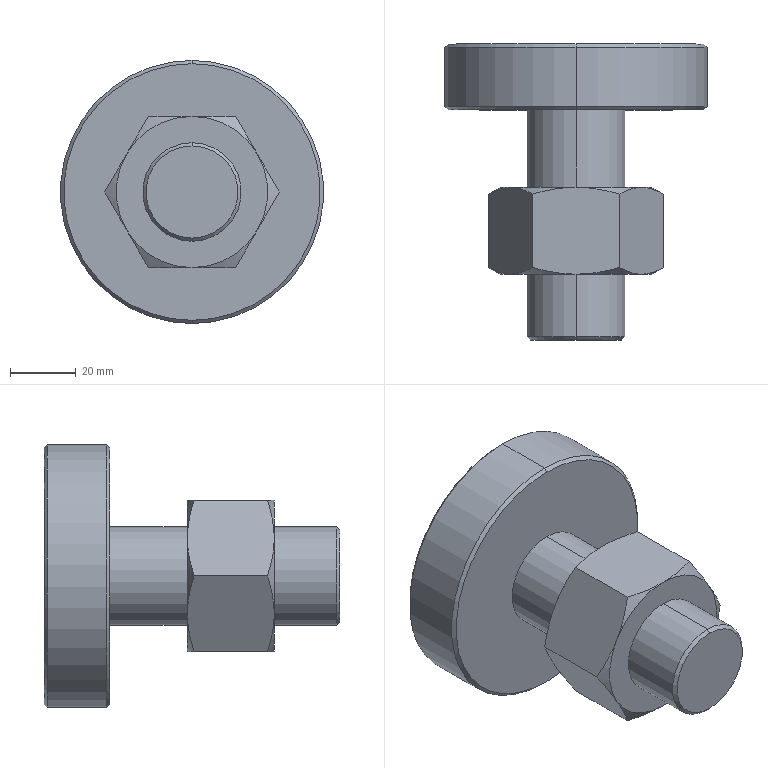Part | SolidWorks | features BaseBody 2 | 2 solids | 35 faces | box 80 x 90 x 80 mm | volume 179222 mm3 | cone 18 | plane 11 | cylinder 6 | commonest cylinder face diameters 30 x4 80 x2
STEP:
#1=CARTESIAN_POINT('',(0.,-70.,-14.));
#2=VERTEX_POINT('',#1);
#3=CARTESIAN_POINT('',(0.,-70.,14.));
#4=VERTEX_POINT('',#3);
#5=CARTESIAN_POINT('',(0.,-70.,0.));
#6=DIRECTION('',(0.,-1.,0.));
#7=DIRECTION('',(0.,0.,1.));
#8=AXIS2_PLACEMENT_3D('',#5,#6,#7);
#9=CIRCLE('',#8,14.);
#10=EDGE_CURVE('',#2,#4,#9,.T.);
#11=ORIENTED_EDGE('',*,*,#10,.F.);
#12=CARTESIAN_POINT('',(0.,-69.,-15.));
#13=VERTEX_POINT('',#12);
#14=CARTESIAN_POINT('',(0.,-69.,-15.));
#15=DIRECTION('',(0.,0.7071,-0.7071));
#16=VECTOR('',#15,1000.);
#17=LINE('',#14,#16);
#18=EDGE_CURVE('',#2,#13,#17,.T.);
#19=ORIENTED_EDGE('',*,*,#18,.T.);
#20=CARTESIAN_POINT('',(0.,-69.,15.));
#21=VERTEX_POINT('',#20);
#22=CARTESIAN_POINT('',(0.,-69.,0.));
#23=DIRECTION('',(0.,1.,0.));
#24=DIRECTION('',(0.,0.,1.));
#25=AXIS2_PLACEMENT_3D('',#22,#23,#24);
#26=CIRCLE('',#25,15.);
#27=EDGE_CURVE('',#21,#13,#26,.T.);
#28=ORIENTED_EDGE('',*,*,#27,.F.);
#29=CARTESIAN_POINT('',(0.,-69.,15.));
#30=DIRECTION('',(0.,0.7071,0.7071));
#31=VECTOR('',#30,1000.);
#32=LINE('',#29,#31);
#33=EDGE_CURVE('',#4,#21,#32,.T.);
#34=ORIENTED_EDGE('',*,*,#33,.F.);
#35=EDGE_LOOP('',(#11,#19,#28,#34));
#36=FACE_OUTER_BOUND('',#35,.T.);
#37=CARTESIAN_POINT('',(0.,-69.,0.));
#38=DIRECTION('',(0.,1.,0.));
#39=DIRECTION('',(0.,0.,1.));
#40=AXIS2_PLACEMENT_3D('',#37,#38,#39);
#41=CONICAL_SURFACE('',#40,15.,0.7854);
#42=ADVANCED_FACE('',(#36),#41,.T.);
#43=CARTESIAN_POINT('',(0.,0.,-39.));
#44=VERTEX_POINT('',#43);
#45=CARTESIAN_POINT('',(0.,0.,39.));
#46=VERTEX_POINT('',#45);
#47=CARTESIAN_POINT('',(0.,0.,0.));
#48=DIRECTION('',(0.,-1.,0.));
#49=DIRECTION('',(0.,0.,1.));
#50=AXIS2_PLACEMENT_3D('',#47,#48,#49);
#51=CIRCLE('',#50,39.);
#52=EDGE_CURVE('',#44,#46,#51,.T.);
#53=ORIENTED_EDGE('',*,*,#52,.F.);
#54=CARTESIAN_POINT('',(0.,1.,-40.));
#55=VERTEX_POINT('',#54);
#56=CARTESIAN_POINT('',(0.,1.,-40.));
#57=DIRECTION('',(0.,0.7071,-0.7071));
#58=VECTOR('',#57,1000.);
#59=LINE('',#56,#58);
#60=EDGE_CURVE('',#44,#55,#59,.T.);
#61=ORIENTED_EDGE('',*,*,#60,.T.);
#62=CARTESIAN_POINT('',(0.,1.,40.));
#63=VERTEX_POINT('',#62);
#64=CARTESIAN_POINT('',(0.,1.,0.));
#65=DIRECTION('',(0.,1.,0.));
#66=DIRECTION('',(0.,0.,1.));
#67=AXIS2_PLACEMENT_3D('',#64,#65,#66);
#68=CIRCLE('',#67,40.);
#69=EDGE_CURVE('',#63,#55,#68,.T.);
#70=ORIENTED_EDGE('',*,*,#69,.F.);
#71=CARTESIAN_POINT('',(0.,1.,40.));
#72=DIRECTION('',(0.,0.7071,0.7071));
#73=VECTOR('',#72,1000.);
#74=LINE('',#71,#73);
#75=EDGE_CURVE('',#46,#63,#74,.T.);
#76=ORIENTED_EDGE('',*,*,#75,.F.);
#77=EDGE_LOOP('',(#53,#61,#70,#76));
#78=FACE_OUTER_BOUND('',#77,.T.);
#79=CARTESIAN_POINT('',(0.,1.,0.));
#80=DIRECTION('',(0.,1.,0.));
#81=DIRECTION('',(0.,0.,1.));
#82=AXIS2_PLACEMENT_3D('',#79,#80,#81);
#83=CONICAL_SURFACE('',#82,40.,0.7854);
#84=ADVANCED_FACE('',(#78),#83,.T.);
#85=CARTESIAN_POINT('',(0.,20.,39.));
#86=VERTEX_POINT('',#85);
#87=CARTESIAN_POINT('',(0.,20.,-39.));
#88=VERTEX_POINT('',#87);
#89=CARTESIAN_POINT('',(0.,20.,0.));
#90=DIRECTION('',(0.,1.,0.));
#91=DIRECTION('',(0.,0.,1.));
#92=AXIS2_PLACEMENT_3D('',#89,#90,#91);
#93=CIRCLE('',#92,39.);
#94=EDGE_CURVE('',#86,#88,#93,.T.);
#95=ORIENTED_EDGE('',*,*,#94,.F.);
#96=CARTESIAN_POINT('',(0.,19.,40.));
#97=VERTEX_POINT('',#96);
#98=CARTESIAN_POINT('',(0.,20.,39.));
#99=DIRECTION('',(0.,-0.7071,0.7071));
#100=VECTOR('',#99,1000.);
#101=LINE('',#98,#100);
#102=EDGE_CURVE('',#86,#97,#101,.T.);
#103=ORIENTED_EDGE('',*,*,#102,.T.);
#104=CARTESIAN_POINT('',(0.,19.,-40.));
#105=VERTEX_POINT('',#104);
#106=CARTESIAN_POINT('',(0.,19.,0.));
#107=DIRECTION('',(0.,-1.,0.));
#108=DIRECTION('',(0.,0.,1.));
#109=AXIS2_PLACEMENT_3D('',#106,#107,#108);
#110=CIRCLE('',#109,40.);
#111=EDGE_CURVE('',#105,#97,#110,.T.);
#112=ORIENTED_EDGE('',*,*,#111,.F.);
#113=CARTESIAN_POINT('',(0.,20.,-39.));
#114=DIRECTION('',(0.,-0.7071,-0.7071));
#115=VECTOR('',#114,1000.);
#116=LINE('',#113,#115);
#117=EDGE_CURVE('',#88,#105,#116,.T.);
#118=ORIENTED_EDGE('',*,*,#117,.F.);
#119=EDGE_LOOP('',(#95,#103,#112,#118));
#120=FACE_OUTER_BOUND('',#119,.T.);
#121=CARTESIAN_POINT('',(0.,20.,0.));
#122=DIRECTION('',(0.,-1.,0.));
#123=DIRECTION('',(0.,0.,-1.));
#124=AXIS2_PLACEMENT_3D('',#121,#122,#123);
#125=CONICAL_SURFACE('',#124,39.,0.7854);
#126=ADVANCED_FACE('',(#120),#125,.T.);
#127=ORIENTED_EDGE('',*,*,#27,.T.);
#128=CARTESIAN_POINT('',(0.,0.,-15.));
#129=VERTEX_POINT('',#128);
#130=CARTESIAN_POINT('',(0.,-70.,-15.));
#131=DIRECTION('',(0.,1.,0.));
#132=VECTOR('',#131,1000.);
#133=LINE('',#130,#132);
#134=EDGE_CURVE('',#13,#129,#133,.T.);
#135=ORIENTED_EDGE('',*,*,#134,.T.);
#136=CARTESIAN_POINT('',(0.,0.,15.));
#137=VERTEX_POINT('',#136);
#138=CARTESIAN_POINT('',(0.,0.,0.));
#139=DIRECTION('',(0.,1.,0.));
#140=DIRECTION('',(0.,0.,1.));
#141=AXIS2_PLACEMENT_3D('',#138,#139,#140);
#142=CIRCLE('',#141,15.);
#143=EDGE_CURVE('',#137,#129,#142,.T.);
#144=ORIENTED_EDGE('',*,*,#143,.F.);
#145=CARTESIAN_POINT('',(0.,-70.,15.));
#146=DIRECTION('',(0.,1.,0.));
#147=VECTOR('',#146,1000.);
#148=LINE('',#145,#147);
#149=EDGE_CURVE('',#21,#137,#148,.T.);
#150=ORIENTED_EDGE('',*,*,#149,.F.);
#151=EDGE_LOOP('',(#127,#135,#144,#150));
#152=FACE_OUTER_BOUND('',#151,.T.);
#153=CARTESIAN_POINT('',(0.,-70.,0.));
#154=DIRECTION('',(0.,1.,0.));
#155=DIRECTION('',(0.,0.,1.));
#156=AXIS2_PLACEMENT_3D('',#153,#154,#155);
#157=CYLINDRICAL_SURFACE('',#156,15.);
#158=ADVANCED_FACE('',(#152),#157,.T.);
#159=ORIENTED_EDGE('',*,*,#111,.T.);
#160=CARTESIAN_POINT('',(0.,20.,40.));
#161=DIRECTION('',(0.,-1.,0.));
#162=VECTOR('',#161,1000.);
#163=LINE('',#160,#162);
#164=EDGE_CURVE('',#97,#63,#163,.T.);
#165=ORIENTED_EDGE('',*,*,#164,.T.);
#166=ORIENTED_EDGE('',*,*,#69,.T.);
#167=CARTESIAN_POINT('',(0.,20.,-40.));
#168=DIRECTION('',(0.,-1.,0.));
#169=VECTOR('',#168,1000.);
#170=LINE('',#167,#169);
#171=EDGE_CURVE('',#105,#55,#170,.T.);
#172=ORIENTED_EDGE('',*,*,#171,.F.);
#173=EDGE_LOOP('',(#159,#165,#166,#172));
#174=FACE_OUTER_BOUND('',#173,.T.);
#175=CARTESIAN_POINT('',(0.,20.,0.));
#176=DIRECTION('',(0.,-1.,0.));
#177=DIRECTION('',(0.,0.,-1.));
#178=AXIS2_PLACEMENT_3D('',#175,#176,#177);
#179=CYLINDRICAL_SURFACE('',#178,40.);
#180=ADVANCED_FACE('',(#174),#179,.T.);
#181=CARTESIAN_POINT('',(0.,20.,0.));
#182=DIRECTION('',(0.,1.,0.));
#183=DIRECTION('',(0.,0.,1.));
#184=AXIS2_PLACEMENT_3D('',#181,#182,#183);
#185=CIRCLE('',#184,39.);
#186=EDGE_CURVE('',#88,#86,#185,.T.);
#187=ORIENTED_EDGE('',*,*,#186,.T.);
#188=ORIENTED_EDGE('',*,*,#94,.T.);
#189=EDGE_LOOP('',(#187,#188));
#190=FACE_OUTER_BOUND('',#189,.T.);
#191=CARTESIAN_POINT('',(0.,20.,0.));
#192=DIRECTION('',(0.,1.,0.));
#193=DIRECTION('',(0.,0.,1.));
#194=AXIS2_PLACEMENT_3D('',#191,#192,#193);
#195=PLANE('',#194);
#196=ADVANCED_FACE('',(#190),#195,.T.);
#197=CARTESIAN_POINT('',(0.,0.,0.));
#198=DIRECTION('',(0.,-1.,0.));
#199=DIRECTION('',(0.,0.,1.));
#200=AXIS2_PLACEMENT_3D('',#197,#198,#199);
#201=CIRCLE('',#200,39.);
#202=EDGE_CURVE('',#46,#44,#201,.T.);
#203=ORIENTED_EDGE('',*,*,#202,.T.);
#204=ORIENTED_EDGE('',*,*,#52,.T.);
#205=EDGE_LOOP('',(#203,#204));
#206=FACE_OUTER_BOUND('',#205,.T.);
#207=ORIENTED_EDGE('',*,*,#143,.T.);
#208=CARTESIAN_POINT('',(0.,0.,0.));
#209=DIRECTION('',(0.,1.,0.));
#210=DIRECTION('',(0.,0.,1.));
#211=AXIS2_PLACEMENT_3D('',#208,#209,#210);
#212=CIRCLE('',#211,15.);
#213=EDGE_CURVE('',#129,#137,#212,.T.);
#214=ORIENTED_EDGE('',*,*,#213,.T.);
#215=EDGE_LOOP('',(#207,#214));
#216=FACE_BOUND('',#215,.T.);
#217=CARTESIAN_POINT('',(0.,0.,0.));
#218=DIRECTION('',(0.,1.,0.));
#219=DIRECTION('',(0.,0.,1.));
#220=AXIS2_PLACEMENT_3D('',#217,#218,#219);
#221=PLANE('',#220);
#222=ADVANCED_FACE('',(#206,#216),#221,.F.);
#223=ORIENTED_EDGE('',*,*,#164,.F.);
#224=CARTESIAN_POINT('',(0.,19.,0.));
#225=DIRECTION('',(0.,-1.,0.));
#226=DIRECTION('',(0.,0.,1.));
#227=AXIS2_PLACEMENT_3D('',#224,#225,#226);
#228=CIRCLE('',#227,40.);
#229=EDGE_CURVE('',#97,#105,#228,.T.);
#230=ORIENTED_EDGE('',*,*,#229,.T.);
#231=ORIENTED_EDGE('',*,*,#171,.T.);
#232=CARTESIAN_POINT('',(0.,1.,0.));
#233=DIRECTION('',(0.,1.,0.));
#234=DIRECTION('',(0.,0.,1.));
#235=AXIS2_PLACEMENT_3D('',#232,#233,#234);
#236=CIRCLE('',#235,40.);
#237=EDGE_CURVE('',#55,#63,#236,.T.);
#238=ORIENTED_EDGE('',*,*,#237,.T.);
#239=EDGE_LOOP('',(#223,#230,#231,#238));
#240=FACE_OUTER_BOUND('',#239,.T.);
#241=CARTESIAN_POINT('',(0.,20.,0.));
#242=DIRECTION('',(0.,-1.,0.));
#243=DIRECTION('',(0.,0.,-1.));
#244=AXIS2_PLACEMENT_3D('',#241,#242,#243);
#245=CYLINDRICAL_SURFACE('',#244,40.);
#246=ADVANCED_FACE('',(#240),#245,.T.);
#247=ORIENTED_EDGE('',*,*,#134,.F.);
#248=CARTESIAN_POINT('',(0.,-69.,0.));
#249=DIRECTION('',(0.,1.,0.));
#250=DIRECTION('',(0.,0.,1.));
#251=AXIS2_PLACEMENT_3D('',#248,#249,#250);
#252=CIRCLE('',#251,15.);
#253=EDGE_CURVE('',#13,#21,#252,.T.);
#254=ORIENTED_EDGE('',*,*,#253,.T.);
#255=ORIENTED_EDGE('',*,*,#149,.T.);
#256=ORIENTED_EDGE('',*,*,#213,.F.);
#257=EDGE_LOOP('',(#247,#254,#255,#256));
#258=FACE_OUTER_BOUND('',#257,.T.);
#259=CARTESIAN_POINT('',(0.,-70.,0.));
#260=DIRECTION('',(0.,1.,0.));
#261=DIRECTION('',(0.,0.,1.));
#262=AXIS2_PLACEMENT_3D('',#259,#260,#261);
#263=CYLINDRICAL_SURFACE('',#262,15.);
#264=ADVANCED_FACE('',(#258),#263,.T.);
#265=CARTESIAN_POINT('',(0.,-70.,0.));
#266=DIRECTION('',(0.,-1.,0.));
#267=DIRECTION('',(0.,0.,1.));
#268=AXIS2_PLACEMENT_3D('',#265,#266,#267);
#269=CIRCLE('',#268,14.);
#270=EDGE_CURVE('',#4,#2,#269,.T.);
#271=ORIENTED_EDGE('',*,*,#270,.T.);
#272=ORIENTED_EDGE('',*,*,#10,.T.);
#273=EDGE_LOOP('',(#271,#272));
#274=FACE_OUTER_BOUND('',#273,.T.);
#275=CARTESIAN_POINT('',(0.,-70.,0.));
#276=DIRECTION('',(0.,1.,0.));
#277=DIRECTION('',(0.,0.,1.));
#278=AXIS2_PLACEMENT_3D('',#275,#276,#277);
#279=PLANE('',#278);
#280=ADVANCED_FACE('',(#274),#279,.F.);
#281=ORIENTED_EDGE('',*,*,#102,.F.);
#282=ORIENTED_EDGE('',*,*,#186,.F.);
#283=ORIENTED_EDGE('',*,*,#117,.T.);
#284=ORIENTED_EDGE('',*,*,#229,.F.);
#285=EDGE_LOOP('',(#281,#282,#283,#284));
#286=FACE_OUTER_BOUND('',#285,.T.);
#287=CARTESIAN_POINT('',(0.,20.,0.));
#288=DIRECTION('',(0.,-1.,0.));
#289=DIRECTION('',(0.,0.,-1.));
#290=AXIS2_PLACEMENT_3D('',#287,#288,#289);
#291=CONICAL_SURFACE('',#290,39.,0.7854);
#292=ADVANCED_FACE('',(#286),#291,.T.);
#293=ORIENTED_EDGE('',*,*,#60,.F.);
#294=ORIENTED_EDGE('',*,*,#202,.F.);
#295=ORIENTED_EDGE('',*,*,#75,.T.);
#296=ORIENTED_EDGE('',*,*,#237,.F.);
#297=EDGE_LOOP('',(#293,#294,#295,#296));
#298=FACE_OUTER_BOUND('',#297,.T.);
#299=CARTESIAN_POINT('',(0.,1.,0.));
#300=DIRECTION('',(0.,1.,0.));
#301=DIRECTION('',(0.,0.,1.));
#302=AXIS2_PLACEMENT_3D('',#299,#300,#301);
#303=CONICAL_SURFACE('',#302,40.,0.7854);
#304=ADVANCED_FACE('',(#298),#303,.T.);
#305=ORIENTED_EDGE('',*,*,#18,.F.);
#306=ORIENTED_EDGE('',*,*,#270,.F.);
#307=ORIENTED_EDGE('',*,*,#33,.T.);
#308=ORIENTED_EDGE('',*,*,#253,.F.);
#309=EDGE_LOOP('',(#305,#306,#307,#308));
#310=FACE_OUTER_BOUND('',#309,.T.);
#311=CARTESIAN_POINT('',(0.,-69.,0.));
#312=DIRECTION('',(0.,1.,0.));
#313=DIRECTION('',(0.,0.,1.));
#314=AXIS2_PLACEMENT_3D('',#311,#312,#313);
#315=CONICAL_SURFACE('',#314,15.,0.7854);
#316=ADVANCED_FACE('',(#310),#315,.T.);
#317=CLOSED_SHELL('',(#42,#84,#126,#158,#180,#196,#222,#246,#264,#280,#292,#304,#316));
#318=MANIFOLD_SOLID_BREP('',#317);
#319=CARTESIAN_POINT('',(0.,-23.6,-15.));
#320=VERTEX_POINT('',#319);
#321=CARTESIAN_POINT('',(0.,-23.6,15.));
#322=VERTEX_POINT('',#321);
#323=CARTESIAN_POINT('',(0.,-23.6,0.));
#324=DIRECTION('',(0.,1.,0.));
#325=DIRECTION('',(0.,0.,1.));
#326=AXIS2_PLACEMENT_3D('',#323,#324,#325);
#327=CIRCLE('',#326,15.);
#328=EDGE_CURVE('',#320,#322,#327,.T.);
#329=ORIENTED_EDGE('',*,*,#328,.T.);
#330=CARTESIAN_POINT('',(0.,-50.,15.));
#331=VERTEX_POINT('',#330);
#332=CARTESIAN_POINT('',(0.,-23.6,15.));
#333=DIRECTION('',(0.,-1.,0.));
#334=VECTOR('',#333,1000.);
#335=LINE('',#332,#334);
#336=EDGE_CURVE('',#322,#331,#335,.T.);
#337=ORIENTED_EDGE('',*,*,#336,.T.);
#338=CARTESIAN_POINT('',(0.,-50.,-15.));
#339=VERTEX_POINT('',#338);
#340=CARTESIAN_POINT('',(0.,-50.,0.));
#341=DIRECTION('',(0.,1.,0.));
#342=DIRECTION('',(0.,0.,1.));
#343=AXIS2_PLACEMENT_3D('',#340,#341,#342);
#344=CIRCLE('',#343,15.);
#345=EDGE_CURVE('',#339,#331,#344,.T.);
#346=ORIENTED_EDGE('',*,*,#345,.F.);
#347=CARTESIAN_POINT('',(0.,-23.6,-15.));
#348=DIRECTION('',(0.,-1.,0.));
#349=VECTOR('',#348,1000.);
#350=LINE('',#347,#349);
#351=EDGE_CURVE('',#320,#339,#350,.T.);
#352=ORIENTED_EDGE('',*,*,#351,.F.);
#353=EDGE_LOOP('',(#329,#337,#346,#352));
#354=FACE_OUTER_BOUND('',#353,.T.);
#355=CARTESIAN_POINT('',(0.,-23.6,0.));
#356=DIRECTION('',(0.,-1.,0.));
#357=DIRECTION('',(0.,0.,-1.));
#358=AXIS2_PLACEMENT_3D('',#355,#356,#357);
#359=CYLINDRICAL_SURFACE('',#358,15.);
#360=ADVANCED_FACE('',(#354),#359,.F.);
#361=ORIENTED_EDGE('',*,*,#328,.F.);
#362=CARTESIAN_POINT('',(0.,-23.6,0.));
#363=DIRECTION('',(0.,1.,0.));
#364=DIRECTION('',(0.,0.,1.));
#365=AXIS2_PLACEMENT_3D('',#362,#363,#364);
#366=CIRCLE('',#365,15.);
#367=EDGE_CURVE('',#322,#320,#366,.T.);
#368=ORIENTED_EDGE('',*,*,#367,.F.);
#369=EDGE_LOOP('',(#361,#368));
#370=FACE_BOUND('',#369,.T.);
#371=CARTESIAN_POINT('',(0.,-23.6,23.));
#372=VERTEX_POINT('',#371);
#373=CARTESIAN_POINT('',(-19.919,-23.6,11.5));
#374=VERTEX_POINT('',#373);
#375=CARTESIAN_POINT('',(0.,-23.6,0.));
#376=DIRECTION('',(0.,-1.,0.));
#377=DIRECTION('',(0.,0.,1.));
#378=AXIS2_PLACEMENT_3D('',#375,#376,#377);
#379=CIRCLE('',#378,23.);
#380=EDGE_CURVE('',#372,#374,#379,.T.);
#381=ORIENTED_EDGE('',*,*,#380,.F.);
#382=CARTESIAN_POINT('',(19.919,-23.6,11.5));
#383=VERTEX_POINT('',#382);
#384=CARTESIAN_POINT('',(0.,-23.6,0.));
#385=DIRECTION('',(0.,-1.,0.));
#386=DIRECTION('',(0.,0.,1.));
#387=AXIS2_PLACEMENT_3D('',#384,#385,#386);
#388=CIRCLE('',#387,23.);
#389=EDGE_CURVE('',#383,#372,#388,.T.);
#390=ORIENTED_EDGE('',*,*,#389,.F.);
#391=CARTESIAN_POINT('',(19.919,-23.6,-11.5));
#392=VERTEX_POINT('',#391);
#393=CARTESIAN_POINT('',(0.,-23.6,0.));
#394=DIRECTION('',(0.,-1.,0.));
#395=DIRECTION('',(0.,0.,1.));
#396=AXIS2_PLACEMENT_3D('',#393,#394,#395);
#397=CIRCLE('',#396,23.);
#398=EDGE_CURVE('',#392,#383,#397,.T.);
#399=ORIENTED_EDGE('',*,*,#398,.F.);
#400=CARTESIAN_POINT('',(0.,-23.6,-23.));
#401=VERTEX_POINT('',#400);
#402=CARTESIAN_POINT('',(0.,-23.6,0.));
#403=DIRECTION('',(0.,-1.,0.));
#404=DIRECTION('',(0.,0.,-1.));
#405=AXIS2_PLACEMENT_3D('',#402,#403,#404);
#406=CIRCLE('',#405,23.);
#407=EDGE_CURVE('',#401,#392,#406,.T.);
#408=ORIENTED_EDGE('',*,*,#407,.F.);
#409=CARTESIAN_POINT('',(-19.919,-23.6,-11.5));
#410=VERTEX_POINT('',#409);
#411=CARTESIAN_POINT('',(0.,-23.6,0.));
#412=DIRECTION('',(0.,-1.,0.));
#413=DIRECTION('',(0.,0.,1.));
#414=AXIS2_PLACEMENT_3D('',#411,#412,#413);
#415=CIRCLE('',#414,23.);
#416=EDGE_CURVE('',#410,#401,#415,.T.);
#417=ORIENTED_EDGE('',*,*,#416,.F.);
#418=CARTESIAN_POINT('',(0.,-23.6,0.));
#419=DIRECTION('',(0.,-1.,0.));
#420=DIRECTION('',(0.,0.,1.));
#421=AXIS2_PLACEMENT_3D('',#418,#419,#420);
#422=CIRCLE('',#421,23.);
#423=EDGE_CURVE('',#374,#410,#422,.T.);
#424=ORIENTED_EDGE('',*,*,#423,.F.);
#425=EDGE_LOOP('',(#381,#390,#399,#408,#417,#424));
#426=FACE_OUTER_BOUND('',#425,.T.);
#427=CARTESIAN_POINT('',(0.,-23.6,0.));
#428=DIRECTION('',(0.,1.,0.));
#429=DIRECTION('',(0.,0.,1.));
#430=AXIS2_PLACEMENT_3D('',#427,#428,#429);
#431=PLANE('',#430);
#432=ADVANCED_FACE('',(#370,#426),#431,.T.);
#433=ORIENTED_EDGE('',*,*,#345,.T.);
#434=CARTESIAN_POINT('',(0.,-50.,0.));
#435=DIRECTION('',(0.,1.,0.));
#436=DIRECTION('',(0.,0.,1.));
#437=AXIS2_PLACEMENT_3D('',#434,#435,#436);
#438=CIRCLE('',#437,15.);
#439=EDGE_CURVE('',#331,#339,#438,.T.);
#440=ORIENTED_EDGE('',*,*,#439,.T.);
#441=EDGE_LOOP('',(#433,#440));
#442=FACE_BOUND('',#441,.T.);
#443=CARTESIAN_POINT('',(19.919,-50.,11.5));
#444=VERTEX_POINT('',#443);
#445=CARTESIAN_POINT('',(0.,-50.,23.));
#446=VERTEX_POINT('',#445);
#447=CARTESIAN_POINT('',(0.,-50.,0.));
#448=DIRECTION('',(0.,-1.,0.));
#449=DIRECTION('',(0.,0.,-1.));
#450=AXIS2_PLACEMENT_3D('',#447,#448,#449);
#451=CIRCLE('',#450,23.);
#452=EDGE_CURVE('',#444,#446,#451,.T.);
#453=ORIENTED_EDGE('',*,*,#452,.T.);
#454=CARTESIAN_POINT('',(-19.919,-50.,11.5));
#455=VERTEX_POINT('',#454);
#456=CARTESIAN_POINT('',(0.,-50.,0.));
#457=DIRECTION('',(0.,-1.,0.));
#458=DIRECTION('',(0.,0.,-1.));
#459=AXIS2_PLACEMENT_3D('',#456,#457,#458);
#460=CIRCLE('',#459,23.);
#461=EDGE_CURVE('',#446,#455,#460,.T.);
#462=ORIENTED_EDGE('',*,*,#461,.T.);
#463=CARTESIAN_POINT('',(-19.919,-50.,-11.5));
#464=VERTEX_POINT('',#463);
#465=CARTESIAN_POINT('',(0.,-50.,0.));
#466=DIRECTION('',(0.,-1.,0.));
#467=DIRECTION('',(0.,0.,-1.));
#468=AXIS2_PLACEMENT_3D('',#465,#466,#467);
#469=CIRCLE('',#468,23.);
#470=EDGE_CURVE('',#455,#464,#469,.T.);
#471=ORIENTED_EDGE('',*,*,#470,.T.);
#472=CARTESIAN_POINT('',(0.,-50.,-23.));
#473=VERTEX_POINT('',#472);
#474=CARTESIAN_POINT('',(0.,-50.,0.));
#475=DIRECTION('',(0.,-1.,0.));
#476=DIRECTION('',(0.,0.,-1.));
#477=AXIS2_PLACEMENT_3D('',#474,#475,#476);
#478=CIRCLE('',#477,23.);
#479=EDGE_CURVE('',#464,#473,#478,.T.);
#480=ORIENTED_EDGE('',*,*,#479,.T.);
#481=CARTESIAN_POINT('',(19.919,-50.,-11.5));
#482=VERTEX_POINT('',#481);
#483=CARTESIAN_POINT('',(0.,-50.,0.));
#484=DIRECTION('',(0.,-1.,0.));
#485=DIRECTION('',(0.,0.,-1.));
#486=AXIS2_PLACEMENT_3D('',#483,#484,#485);
#487=CIRCLE('',#486,23.);
#488=EDGE_CURVE('',#473,#482,#487,.T.);
#489=ORIENTED_EDGE('',*,*,#488,.T.);
#490=CARTESIAN_POINT('',(0.,-50.,0.));
#491=DIRECTION('',(0.,-1.,0.));
#492=DIRECTION('',(0.,0.,-1.));
#493=AXIS2_PLACEMENT_3D('',#490,#491,#492);
#494=CIRCLE('',#493,23.);
#495=EDGE_CURVE('',#482,#444,#494,.T.);
#496=ORIENTED_EDGE('',*,*,#495,.T.);
#497=EDGE_LOOP('',(#453,#462,#471,#480,#489,#496));
#498=FACE_OUTER_BOUND('',#497,.T.);
#499=CARTESIAN_POINT('',(0.,-50.,0.));
#500=DIRECTION('',(0.,1.,0.));
#501=DIRECTION('',(0.,0.,1.));
#502=AXIS2_PLACEMENT_3D('',#499,#500,#501);
#503=PLANE('',#502);
#504=ADVANCED_FACE('',(#442,#498),#503,.F.);
#505=CARTESIAN_POINT('',(26.558,-25.654,0.));
#506=VERTEX_POINT('',#505);
#507=CARTESIAN_POINT('',(26.558,-47.946,0.));
#508=VERTEX_POINT('',#507);
#509=CARTESIAN_POINT('',(26.558,-23.6,0.));
#510=DIRECTION('',(0.,-1.,0.));
#511=VECTOR('',#510,1000.);
#512=LINE('',#509,#511);
#513=EDGE_CURVE('',#506,#508,#512,.T.);
#514=ORIENTED_EDGE('',*,*,#513,.F.);
#515=CARTESIAN_POINT('',(26.558,-25.654,0.));
#516=CARTESIAN_POINT('',(25.472,-25.027,1.881));
#517=CARTESIAN_POINT('',(24.378,-24.511,3.776));
#518=CARTESIAN_POINT('',(22.167,-23.796,7.606));
#519=CARTESIAN_POINT('',(21.05,-23.6,9.541));
#520=CARTESIAN_POINT('',(19.919,-23.6,11.5));
#521=B_SPLINE_CURVE_WITH_KNOTS('',3,(#515,#516,#517,#518,#519,#520),.UNSPECIFIED.,.F.,.F.,(4,2,4),(0.000000238,0.006718,0.01344),.UNSPECIFIED.);
#522=EDGE_CURVE('',#506,#383,#521,.T.);
#523=ORIENTED_EDGE('',*,*,#522,.T.);
#524=CARTESIAN_POINT('',(13.279,-25.654,23.));
#525=VERTEX_POINT('',#524);
#526=CARTESIAN_POINT('',(19.919,-23.6,11.5));
#527=CARTESIAN_POINT('',(19.637,-23.6,11.988));
#528=CARTESIAN_POINT('',(19.354,-23.612,12.478));
#529=CARTESIAN_POINT('',(18.79,-23.66,13.455));
#530=CARTESIAN_POINT('',(18.509,-23.696,13.941));
#531=CARTESIAN_POINT('',(17.669,-23.836,15.396));
#532=CARTESIAN_POINT('',(17.113,-23.976,16.359));
#533=CARTESIAN_POINT('',(15.455,-24.512,19.231));
#534=CARTESIAN_POINT('',(14.362,-25.029,21.123));
#535=CARTESIAN_POINT('',(13.279,-25.654,23.));
#536=B_SPLINE_CURVE_WITH_KNOTS('',3,(#526,#527,#528,#529,#530,#531,#532,#533,#534,#535),.UNSPECIFIED.,.F.,.F.,(4,2,2,2,4),(0.01344,0.01511,0.01678,0.02013,0.02682),.UNSPECIFIED.);
#537=EDGE_CURVE('',#383,#525,#536,.T.);
#538=ORIENTED_EDGE('',*,*,#537,.T.);
#539=CARTESIAN_POINT('',(13.279,-47.946,23.));
#540=VERTEX_POINT('',#539);
#541=CARTESIAN_POINT('',(13.279,-23.6,23.));
#542=DIRECTION('',(0.,-1.,0.));
#543=VECTOR('',#542,1000.);
#544=LINE('',#541,#543);
#545=EDGE_CURVE('',#525,#540,#544,.T.);
#546=ORIENTED_EDGE('',*,*,#545,.T.);
#547=CARTESIAN_POINT('',(19.919,-50.,11.5));
#548=CARTESIAN_POINT('',(19.637,-50.,11.988));
#549=CARTESIAN_POINT('',(19.354,-49.988,12.478));
#550=CARTESIAN_POINT('',(18.79,-49.94,13.455));
#551=CARTESIAN_POINT('',(18.509,-49.904,13.941));
#552=CARTESIAN_POINT('',(17.669,-49.764,15.396));
#553=CARTESIAN_POINT('',(17.113,-49.624,16.359));
#554=CARTESIAN_POINT('',(15.455,-49.088,19.231));
#555=CARTESIAN_POINT('',(14.362,-48.571,21.123));
#556=CARTESIAN_POINT('',(13.279,-47.946,23.));
#557=B_SPLINE_CURVE_WITH_KNOTS('',3,(#547,#548,#549,#550,#551,#552,#553,#554,#555,#556),.UNSPECIFIED.,.F.,.F.,(4,2,2,2,4),(0.01344,0.01511,0.01678,0.02013,0.02682),.UNSPECIFIED.);
#558=EDGE_CURVE('',#444,#540,#557,.T.);
#559=ORIENTED_EDGE('',*,*,#558,.F.);
#560=CARTESIAN_POINT('',(26.558,-47.946,0.));
#561=CARTESIAN_POINT('',(25.472,-48.573,1.881));
#562=CARTESIAN_POINT('',(24.378,-49.089,3.776));
#563=CARTESIAN_POINT('',(22.167,-49.804,7.606));
#564=CARTESIAN_POINT('',(21.05,-50.,9.541));
#565=CARTESIAN_POINT('',(19.919,-50.,11.5));
#566=B_SPLINE_CURVE_WITH_KNOTS('',3,(#560,#561,#562,#563,#564,#565),.UNSPECIFIED.,.F.,.F.,(4,2,4),(0.000000238,0.006718,0.01344),.UNSPECIFIED.);
#567=EDGE_CURVE('',#508,#444,#566,.T.);
#568=ORIENTED_EDGE('',*,*,#567,.F.);
#569=EDGE_LOOP('',(#514,#523,#538,#546,#559,#568));
#570=FACE_OUTER_BOUND('',#569,.T.);
#571=CARTESIAN_POINT('',(13.279,-23.6,23.));
#572=DIRECTION('',(-0.866,0.,-0.5));
#573=DIRECTION('',(-0.5,0.,0.866));
#574=AXIS2_PLACEMENT_3D('',#571,#572,#573);
#575=PLANE('',#574);
#576=ADVANCED_FACE('',(#570),#575,.F.);
#577=CARTESIAN_POINT('',(13.279,-25.654,-23.));
#578=VERTEX_POINT('',#577);
#579=CARTESIAN_POINT('',(13.279,-47.946,-23.));
#580=VERTEX_POINT('',#579);
#581=CARTESIAN_POINT('',(13.279,-23.6,-23.));
#582=DIRECTION('',(0.,-1.,0.));
#583=VECTOR('',#582,1000.);
#584=LINE('',#581,#583);
#585=EDGE_CURVE('',#578,#580,#584,.T.);
#586=ORIENTED_EDGE('',*,*,#585,.F.);
#587=CARTESIAN_POINT('',(13.279,-25.654,-23.));
#588=CARTESIAN_POINT('',(14.365,-25.027,-21.119));
#589=CARTESIAN_POINT('',(15.459,-24.511,-19.224));
#590=CARTESIAN_POINT('',(17.67,-23.796,-15.394));
#591=CARTESIAN_POINT('',(18.787,-23.6,-13.459));
#592=CARTESIAN_POINT('',(19.919,-23.6,-11.5));
#593=B_SPLINE_CURVE_WITH_KNOTS('',3,(#587,#588,#589,#590,#591,#592),.UNSPECIFIED.,.F.,.F.,(4,2,4),(0.000000238,0.006718,0.01344),.UNSPECIFIED.);
#594=EDGE_CURVE('',#578,#392,#593,.T.);
#595=ORIENTED_EDGE('',*,*,#594,.T.);
#596=CARTESIAN_POINT('',(19.919,-23.6,-11.5));
#597=CARTESIAN_POINT('',(20.2,-23.6,-11.012));
#598=CARTESIAN_POINT('',(20.483,-23.612,-10.522));
#599=CARTESIAN_POINT('',(21.047,-23.66,-9.545));
#600=CARTESIAN_POINT('',(21.328,-23.696,-9.059));
#601=CARTESIAN_POINT('',(22.168,-23.836,-7.604));
#602=CARTESIAN_POINT('',(22.724,-23.976,-6.641));
#603=CARTESIAN_POINT('',(24.382,-24.512,-3.769));
#604=CARTESIAN_POINT('',(25.475,-25.029,-1.877));
#605=CARTESIAN_POINT('',(26.558,-25.654,0.));
#606=B_SPLINE_CURVE_WITH_KNOTS('',3,(#596,#597,#598,#599,#600,#601,#602,#603,#604,#605),.UNSPECIFIED.,.F.,.F.,(4,2,2,2,4),(0.01344,0.01511,0.01678,0.02013,0.02682),.UNSPECIFIED.);
#607=EDGE_CURVE('',#392,#506,#606,.T.);
#608=ORIENTED_EDGE('',*,*,#607,.T.);
#609=ORIENTED_EDGE('',*,*,#513,.T.);
#610=CARTESIAN_POINT('',(19.919,-50.,-11.5));
#611=CARTESIAN_POINT('',(20.2,-50.,-11.012));
#612=CARTESIAN_POINT('',(20.483,-49.988,-10.522));
#613=CARTESIAN_POINT('',(21.047,-49.94,-9.545));
#614=CARTESIAN_POINT('',(21.328,-49.904,-9.059));
#615=CARTESIAN_POINT('',(22.168,-49.764,-7.604));
#616=CARTESIAN_POINT('',(22.724,-49.624,-6.641));
#617=CARTESIAN_POINT('',(24.382,-49.088,-3.769));
#618=CARTESIAN_POINT('',(25.475,-48.571,-1.877));
#619=CARTESIAN_POINT('',(26.558,-47.946,0.));
#620=B_SPLINE_CURVE_WITH_KNOTS('',3,(#610,#611,#612,#613,#614,#615,#616,#617,#618,#619),.UNSPECIFIED.,.F.,.F.,(4,2,2,2,4),(0.01344,0.01511,0.01678,0.02013,0.02682),.UNSPECIFIED.);
#621=EDGE_CURVE('',#482,#508,#620,.T.);
#622=ORIENTED_EDGE('',*,*,#621,.F.);
#623=CARTESIAN_POINT('',(13.279,-47.946,-23.));
#624=CARTESIAN_POINT('',(14.365,-48.573,-21.119));
#625=CARTESIAN_POINT('',(15.459,-49.089,-19.224));
#626=CARTESIAN_POINT('',(17.67,-49.804,-15.394));
#627=CARTESIAN_POINT('',(18.787,-50.,-13.459));
#628=CARTESIAN_POINT('',(19.919,-50.,-11.5));
#629=B_SPLINE_CURVE_WITH_KNOTS('',3,(#623,#624,#625,#626,#627,#628),.UNSPECIFIED.,.F.,.F.,(4,2,4),(0.000000238,0.006718,0.01344),.UNSPECIFIED.);
#630=EDGE_CURVE('',#580,#482,#629,.T.);
#631=ORIENTED_EDGE('',*,*,#630,.F.);
#632=EDGE_LOOP('',(#586,#595,#608,#609,#622,#631));
#633=FACE_OUTER_BOUND('',#632,.T.);
#634=CARTESIAN_POINT('',(26.558,-23.6,0.));
#635=DIRECTION('',(-0.866,0.,0.5));
#636=DIRECTION('',(0.5,0.,0.866));
#637=AXIS2_PLACEMENT_3D('',#634,#635,#636);
#638=PLANE('',#637);
#639=ADVANCED_FACE('',(#633),#638,.F.);
#640=CARTESIAN_POINT('',(-13.279,-25.654,-23.));
#641=VERTEX_POINT('',#640);
#642=CARTESIAN_POINT('',(-13.279,-47.946,-23.));
#643=VERTEX_POINT('',#642);
#644=CARTESIAN_POINT('',(-13.279,-23.6,-23.));
#645=DIRECTION('',(0.,-1.,0.));
#646=VECTOR('',#645,1000.);
#647=LINE('',#644,#646);
#648=EDGE_CURVE('',#641,#643,#647,.T.);
#649=ORIENTED_EDGE('',*,*,#648,.F.);
#650=CARTESIAN_POINT('',(-13.279,-25.654,-23.));
#651=CARTESIAN_POINT('',(-11.116,-25.03,-23.));
#652=CARTESIAN_POINT('',(-8.934,-24.514,-23.));
#653=CARTESIAN_POINT('',(-4.513,-23.798,-23.));
#654=CARTESIAN_POINT('',(-2.274,-23.6,-23.));
#655=CARTESIAN_POINT('',(0.,-23.6,-23.));
#656=B_SPLINE_CURVE_WITH_KNOTS('',3,(#650,#651,#652,#653,#654,#655),.UNSPECIFIED.,.F.,.F.,(4,2,4),(0.02897,0.03573,0.04248),.UNSPECIFIED.);
#657=EDGE_CURVE('',#641,#401,#656,.T.);
#658=ORIENTED_EDGE('',*,*,#657,.T.);
#659=CARTESIAN_POINT('',(0.,-23.6,-23.));
#660=CARTESIAN_POINT('',(1.136,-23.6,-23.));
#661=CARTESIAN_POINT('',(2.268,-23.649,-23.));
#662=CARTESIAN_POINT('',(4.51,-23.838,-23.));
#663=CARTESIAN_POINT('',(5.622,-23.977,-23.));
#664=CARTESIAN_POINT('',(8.938,-24.515,-23.));
#665=CARTESIAN_POINT('',(11.118,-25.031,-23.));
#666=CARTESIAN_POINT('',(13.279,-25.654,-23.));
#667=B_SPLINE_CURVE_WITH_KNOTS('',3,(#659,#660,#661,#662,#663,#664,#665,#666),.UNSPECIFIED.,.F.,.F.,(4,2,2,4),(0.04248,0.04586,0.04923,0.05599),.UNSPECIFIED.);
#668=EDGE_CURVE('',#401,#578,#667,.T.);
#669=ORIENTED_EDGE('',*,*,#668,.T.);
#670=ORIENTED_EDGE('',*,*,#585,.T.);
#671=CARTESIAN_POINT('',(0.,-50.,-23.));
#672=CARTESIAN_POINT('',(1.136,-50.,-23.));
#673=CARTESIAN_POINT('',(2.268,-49.951,-23.));
#674=CARTESIAN_POINT('',(4.51,-49.762,-23.));
#675=CARTESIAN_POINT('',(5.622,-49.623,-23.));
#676=CARTESIAN_POINT('',(8.938,-49.085,-23.));
#677=CARTESIAN_POINT('',(11.118,-48.569,-23.));
#678=CARTESIAN_POINT('',(13.279,-47.946,-23.));
#679=B_SPLINE_CURVE_WITH_KNOTS('',3,(#671,#672,#673,#674,#675,#676,#677,#678),.UNSPECIFIED.,.F.,.F.,(4,2,2,4),(0.04248,0.04586,0.04923,0.05599),.UNSPECIFIED.);
#680=EDGE_CURVE('',#473,#580,#679,.T.);
#681=ORIENTED_EDGE('',*,*,#680,.F.);
#682=CARTESIAN_POINT('',(-13.279,-47.946,-23.));
#683=CARTESIAN_POINT('',(-11.116,-48.57,-23.));
#684=CARTESIAN_POINT('',(-8.934,-49.086,-23.));
#685=CARTESIAN_POINT('',(-4.513,-49.802,-23.));
#686=CARTESIAN_POINT('',(-2.274,-50.,-23.));
#687=CARTESIAN_POINT('',(0.,-50.,-23.));
#688=B_SPLINE_CURVE_WITH_KNOTS('',3,(#682,#683,#684,#685,#686,#687),.UNSPECIFIED.,.F.,.F.,(4,2,4),(0.02897,0.03573,0.04248),.UNSPECIFIED.);
#689=EDGE_CURVE('',#643,#473,#688,.T.);
#690=ORIENTED_EDGE('',*,*,#689,.F.);
#691=EDGE_LOOP('',(#649,#658,#669,#670,#681,#690));
#692=FACE_OUTER_BOUND('',#691,.T.);
#693=CARTESIAN_POINT('',(13.279,-23.6,-23.));
#694=DIRECTION('',(0.,0.,1.));
#695=DIRECTION('',(1.,0.,0.));
#696=AXIS2_PLACEMENT_3D('',#693,#694,#695);
#697=PLANE('',#696);
#698=ADVANCED_FACE('',(#692),#697,.F.);
#699=CARTESIAN_POINT('',(-26.558,-25.654,0.));
#700=VERTEX_POINT('',#699);
#701=CARTESIAN_POINT('',(-26.558,-47.946,0.));
#702=VERTEX_POINT('',#701);
#703=CARTESIAN_POINT('',(-26.558,-23.6,0.));
#704=DIRECTION('',(0.,-1.,0.));
#705=VECTOR('',#704,1000.);
#706=LINE('',#703,#705);
#707=EDGE_CURVE('',#700,#702,#706,.T.);
#708=ORIENTED_EDGE('',*,*,#707,.F.);
#709=CARTESIAN_POINT('',(-26.558,-25.654,0.));
#710=CARTESIAN_POINT('',(-25.472,-25.027,-1.881));
#711=CARTESIAN_POINT('',(-24.378,-24.511,-3.776));
#712=CARTESIAN_POINT('',(-22.167,-23.796,-7.606));
#713=CARTESIAN_POINT('',(-21.05,-23.6,-9.541));
#714=CARTESIAN_POINT('',(-19.919,-23.6,-11.5));
#715=B_SPLINE_CURVE_WITH_KNOTS('',3,(#709,#710,#711,#712,#713,#714),.UNSPECIFIED.,.F.,.F.,(4,2,4),(0.000000238,0.006718,0.01344),.UNSPECIFIED.);
#716=EDGE_CURVE('',#700,#410,#715,.T.);
#717=ORIENTED_EDGE('',*,*,#716,.T.);
#718=CARTESIAN_POINT('',(-19.919,-23.6,-11.5));
#719=CARTESIAN_POINT('',(-19.637,-23.6,-11.988));
#720=CARTESIAN_POINT('',(-19.354,-23.612,-12.478));
#721=CARTESIAN_POINT('',(-18.79,-23.66,-13.455));
#722=CARTESIAN_POINT('',(-18.509,-23.696,-13.941));
#723=CARTESIAN_POINT('',(-17.669,-23.836,-15.396));
#724=CARTESIAN_POINT('',(-17.113,-23.976,-16.359));
#725=CARTESIAN_POINT('',(-15.455,-24.512,-19.231));
#726=CARTESIAN_POINT('',(-14.362,-25.029,-21.123));
#727=CARTESIAN_POINT('',(-13.279,-25.654,-23.));
#728=B_SPLINE_CURVE_WITH_KNOTS('',3,(#718,#719,#720,#721,#722,#723,#724,#725,#726,#727),.UNSPECIFIED.,.F.,.F.,(4,2,2,2,4),(0.01344,0.01511,0.01678,0.02013,0.02682),.UNSPECIFIED.);
#729=EDGE_CURVE('',#410,#641,#728,.T.);
#730=ORIENTED_EDGE('',*,*,#729,.T.);
#731=ORIENTED_EDGE('',*,*,#648,.T.);
#732=CARTESIAN_POINT('',(-19.919,-50.,-11.5));
#733=CARTESIAN_POINT('',(-19.637,-50.,-11.988));
#734=CARTESIAN_POINT('',(-19.354,-49.988,-12.478));
#735=CARTESIAN_POINT('',(-18.79,-49.94,-13.455));
#736=CARTESIAN_POINT('',(-18.509,-49.904,-13.941));
#737=CARTESIAN_POINT('',(-17.669,-49.764,-15.396));
#738=CARTESIAN_POINT('',(-17.113,-49.624,-16.359));
#739=CARTESIAN_POINT('',(-15.455,-49.088,-19.231));
#740=CARTESIAN_POINT('',(-14.362,-48.571,-21.123));
#741=CARTESIAN_POINT('',(-13.279,-47.946,-23.));
#742=B_SPLINE_CURVE_WITH_KNOTS('',3,(#732,#733,#734,#735,#736,#737,#738,#739,#740,#741),.UNSPECIFIED.,.F.,.F.,(4,2,2,2,4),(0.01344,0.01511,0.01678,0.02013,0.02682),.UNSPECIFIED.);
#743=EDGE_CURVE('',#464,#643,#742,.T.);
#744=ORIENTED_EDGE('',*,*,#743,.F.);
#745=CARTESIAN_POINT('',(-26.558,-47.946,0.));
#746=CARTESIAN_POINT('',(-25.472,-48.573,-1.881));
#747=CARTESIAN_POINT('',(-24.378,-49.089,-3.776));
#748=CARTESIAN_POINT('',(-22.167,-49.804,-7.606));
#749=CARTESIAN_POINT('',(-21.05,-50.,-9.541));
#750=CARTESIAN_POINT('',(-19.919,-50.,-11.5));
#751=B_SPLINE_CURVE_WITH_KNOTS('',3,(#745,#746,#747,#748,#749,#750),.UNSPECIFIED.,.F.,.F.,(4,2,4),(0.000000238,0.006718,0.01344),.UNSPECIFIED.);
#752=EDGE_CURVE('',#702,#464,#751,.T.);
#753=ORIENTED_EDGE('',*,*,#752,.F.);
#754=EDGE_LOOP('',(#708,#717,#730,#731,#744,#753));
#755=FACE_OUTER_BOUND('',#754,.T.);
#756=CARTESIAN_POINT('',(-13.279,-23.6,-23.));
#757=DIRECTION('',(0.866,0.,0.5));
#758=DIRECTION('',(0.5,0.,-0.866));
#759=AXIS2_PLACEMENT_3D('',#756,#757,#758);
#760=PLANE('',#759);
#761=ADVANCED_FACE('',(#755),#760,.F.);
#762=CARTESIAN_POINT('',(-13.279,-25.654,23.));
#763=VERTEX_POINT('',#762);
#764=CARTESIAN_POINT('',(-13.279,-47.946,23.));
#765=VERTEX_POINT('',#764);
#766=CARTESIAN_POINT('',(-13.279,-23.6,23.));
#767=DIRECTION('',(0.,-1.,0.));
#768=VECTOR('',#767,1000.);
#769=LINE('',#766,#768);
#770=EDGE_CURVE('',#763,#765,#769,.T.);
#771=ORIENTED_EDGE('',*,*,#770,.F.);
#772=CARTESIAN_POINT('',(-13.279,-25.654,23.));
#773=CARTESIAN_POINT('',(-14.365,-25.027,21.119));
#774=CARTESIAN_POINT('',(-15.459,-24.511,19.224));
#775=CARTESIAN_POINT('',(-17.67,-23.796,15.394));
#776=CARTESIAN_POINT('',(-18.787,-23.6,13.459));
#777=CARTESIAN_POINT('',(-19.919,-23.6,11.5));
#778=B_SPLINE_CURVE_WITH_KNOTS('',3,(#772,#773,#774,#775,#776,#777),.UNSPECIFIED.,.F.,.F.,(4,2,4),(0.000000238,0.006718,0.01344),.UNSPECIFIED.);
#779=EDGE_CURVE('',#763,#374,#778,.T.);
#780=ORIENTED_EDGE('',*,*,#779,.T.);
#781=CARTESIAN_POINT('',(-19.919,-23.6,11.5));
#782=CARTESIAN_POINT('',(-20.2,-23.6,11.012));
#783=CARTESIAN_POINT('',(-20.483,-23.612,10.522));
#784=CARTESIAN_POINT('',(-21.047,-23.66,9.545));
#785=CARTESIAN_POINT('',(-21.328,-23.696,9.059));
#786=CARTESIAN_POINT('',(-22.168,-23.836,7.604));
#787=CARTESIAN_POINT('',(-22.724,-23.976,6.641));
#788=CARTESIAN_POINT('',(-24.382,-24.512,3.769));
#789=CARTESIAN_POINT('',(-25.475,-25.029,1.877));
#790=CARTESIAN_POINT('',(-26.558,-25.654,0.));
#791=B_SPLINE_CURVE_WITH_KNOTS('',3,(#781,#782,#783,#784,#785,#786,#787,#788,#789,#790),.UNSPECIFIED.,.F.,.F.,(4,2,2,2,4),(0.01344,0.01511,0.01678,0.02013,0.02682),.UNSPECIFIED.);
#792=EDGE_CURVE('',#374,#700,#791,.T.);
#793=ORIENTED_EDGE('',*,*,#792,.T.);
#794=ORIENTED_EDGE('',*,*,#707,.T.);
#795=CARTESIAN_POINT('',(-19.919,-50.,11.5));
#796=CARTESIAN_POINT('',(-20.2,-50.,11.012));
#797=CARTESIAN_POINT('',(-20.483,-49.988,10.522));
#798=CARTESIAN_POINT('',(-21.047,-49.94,9.545));
#799=CARTESIAN_POINT('',(-21.328,-49.904,9.059));
#800=CARTESIAN_POINT('',(-22.168,-49.764,7.604));
#801=CARTESIAN_POINT('',(-22.724,-49.624,6.641));
#802=CARTESIAN_POINT('',(-24.382,-49.088,3.769));
#803=CARTESIAN_POINT('',(-25.475,-48.571,1.877));
#804=CARTESIAN_POINT('',(-26.558,-47.946,0.));
#805=B_SPLINE_CURVE_WITH_KNOTS('',3,(#795,#796,#797,#798,#799,#800,#801,#802,#803,#804),.UNSPECIFIED.,.F.,.F.,(4,2,2,2,4),(0.01344,0.01511,0.01678,0.02013,0.02682),.UNSPECIFIED.);
#806=EDGE_CURVE('',#455,#702,#805,.T.);
#807=ORIENTED_EDGE('',*,*,#806,.F.);
#808=CARTESIAN_POINT('',(-13.279,-47.946,23.));
#809=CARTESIAN_POINT('',(-14.365,-48.573,21.119));
#810=CARTESIAN_POINT('',(-15.459,-49.089,19.224));
#811=CARTESIAN_POINT('',(-17.67,-49.804,15.394));
#812=CARTESIAN_POINT('',(-18.787,-50.,13.459));
#813=CARTESIAN_POINT('',(-19.919,-50.,11.5));
#814=B_SPLINE_CURVE_WITH_KNOTS('',3,(#808,#809,#810,#811,#812,#813),.UNSPECIFIED.,.F.,.F.,(4,2,4),(0.000000238,0.006718,0.01344),.UNSPECIFIED.);
#815=EDGE_CURVE('',#765,#455,#814,.T.);
#816=ORIENTED_EDGE('',*,*,#815,.F.);
#817=EDGE_LOOP('',(#771,#780,#793,#794,#807,#816));
#818=FACE_OUTER_BOUND('',#817,.T.);
#819=CARTESIAN_POINT('',(-26.558,-23.6,0.));
#820=DIRECTION('',(0.866,0.,-0.5));
#821=DIRECTION('',(-0.5,0.,-0.866));
#822=AXIS2_PLACEMENT_3D('',#819,#820,#821);
#823=PLANE('',#822);
#824=ADVANCED_FACE('',(#818),#823,.F.);
#825=ORIENTED_EDGE('',*,*,#545,.F.);
#826=CARTESIAN_POINT('',(13.279,-25.654,23.));
#827=CARTESIAN_POINT('',(11.116,-25.03,23.));
#828=CARTESIAN_POINT('',(8.934,-24.514,23.));
#829=CARTESIAN_POINT('',(4.513,-23.798,23.));
#830=CARTESIAN_POINT('',(2.274,-23.6,23.));
#831=CARTESIAN_POINT('',(0.,-23.6,23.));
#832=B_SPLINE_CURVE_WITH_KNOTS('',3,(#826,#827,#828,#829,#830,#831),.UNSPECIFIED.,.F.,.F.,(4,2,4),(0.02897,0.03573,0.04248),.UNSPECIFIED.);
#833=EDGE_CURVE('',#525,#372,#832,.T.);
#834=ORIENTED_EDGE('',*,*,#833,.T.);
#835=CARTESIAN_POINT('',(0.,-23.6,23.));
#836=CARTESIAN_POINT('',(-1.136,-23.6,23.));
#837=CARTESIAN_POINT('',(-2.268,-23.649,23.));
#838=CARTESIAN_POINT('',(-4.51,-23.838,23.));
#839=CARTESIAN_POINT('',(-5.622,-23.977,23.));
#840=CARTESIAN_POINT('',(-8.938,-24.515,23.));
#841=CARTESIAN_POINT('',(-11.118,-25.031,23.));
#842=CARTESIAN_POINT('',(-13.279,-25.654,23.));
#843=B_SPLINE_CURVE_WITH_KNOTS('',3,(#835,#836,#837,#838,#839,#840,#841,#842),.UNSPECIFIED.,.F.,.F.,(4,2,2,4),(0.04248,0.04586,0.04923,0.05599),.UNSPECIFIED.);
#844=EDGE_CURVE('',#372,#763,#843,.T.);
#845=ORIENTED_EDGE('',*,*,#844,.T.);
#846=ORIENTED_EDGE('',*,*,#770,.T.);
#847=CARTESIAN_POINT('',(0.,-50.,23.));
#848=CARTESIAN_POINT('',(-1.136,-50.,23.));
#849=CARTESIAN_POINT('',(-2.268,-49.951,23.));
#850=CARTESIAN_POINT('',(-4.51,-49.762,23.));
#851=CARTESIAN_POINT('',(-5.622,-49.623,23.));
#852=CARTESIAN_POINT('',(-8.938,-49.085,23.));
#853=CARTESIAN_POINT('',(-11.118,-48.569,23.));
#854=CARTESIAN_POINT('',(-13.279,-47.946,23.));
#855=B_SPLINE_CURVE_WITH_KNOTS('',3,(#847,#848,#849,#850,#851,#852,#853,#854),.UNSPECIFIED.,.F.,.F.,(4,2,2,4),(0.04248,0.04586,0.04923,0.05599),.UNSPECIFIED.);
#856=EDGE_CURVE('',#446,#765,#855,.T.);
#857=ORIENTED_EDGE('',*,*,#856,.F.);
#858=CARTESIAN_POINT('',(13.279,-47.946,23.));
#859=CARTESIAN_POINT('',(11.116,-48.57,23.));
#860=CARTESIAN_POINT('',(8.934,-49.086,23.));
#861=CARTESIAN_POINT('',(4.513,-49.802,23.));
#862=CARTESIAN_POINT('',(2.274,-50.,23.));
#863=CARTESIAN_POINT('',(0.,-50.,23.));
#864=B_SPLINE_CURVE_WITH_KNOTS('',3,(#858,#859,#860,#861,#862,#863),.UNSPECIFIED.,.F.,.F.,(4,2,4),(0.02897,0.03573,0.04248),.UNSPECIFIED.);
#865=EDGE_CURVE('',#540,#446,#864,.T.);
#866=ORIENTED_EDGE('',*,*,#865,.F.);
#867=EDGE_LOOP('',(#825,#834,#845,#846,#857,#866));
#868=FACE_OUTER_BOUND('',#867,.T.);
#869=CARTESIAN_POINT('',(-13.279,-23.6,23.));
#870=DIRECTION('',(0.,0.,-1.));
#871=DIRECTION('',(-1.,0.,0.));
#872=AXIS2_PLACEMENT_3D('',#869,#870,#871);
#873=PLANE('',#872);
#874=ADVANCED_FACE('',(#868),#873,.F.);
#875=ORIENTED_EDGE('',*,*,#336,.F.);
#876=ORIENTED_EDGE('',*,*,#367,.T.);
#877=ORIENTED_EDGE('',*,*,#351,.T.);
#878=ORIENTED_EDGE('',*,*,#439,.F.);
#879=EDGE_LOOP('',(#875,#876,#877,#878));
#880=FACE_OUTER_BOUND('',#879,.T.);
#881=CARTESIAN_POINT('',(0.,-23.6,0.));
#882=DIRECTION('',(0.,-1.,0.));
#883=DIRECTION('',(0.,0.,-1.));
#884=AXIS2_PLACEMENT_3D('',#881,#882,#883);
#885=CYLINDRICAL_SURFACE('',#884,15.);
#886=ADVANCED_FACE('',(#880),#885,.F.);
#887=ORIENTED_EDGE('',*,*,#815,.T.);
#888=ORIENTED_EDGE('',*,*,#461,.F.);
#889=ORIENTED_EDGE('',*,*,#856,.T.);
#890=EDGE_LOOP('',(#887,#888,#889));
#891=FACE_OUTER_BOUND('',#890,.T.);
#892=CARTESIAN_POINT('',(0.,-50.,0.));
#893=DIRECTION('',(0.,1.,0.));
#894=DIRECTION('',(0.,0.,-1.));
#895=AXIS2_PLACEMENT_3D('',#892,#893,#894);
#896=CONICAL_SURFACE('',#895,23.,1.047);
#897=ADVANCED_FACE('',(#891),#896,.T.);
#898=ORIENTED_EDGE('',*,*,#558,.T.);
#899=ORIENTED_EDGE('',*,*,#865,.T.);
#900=ORIENTED_EDGE('',*,*,#452,.F.);
#901=EDGE_LOOP('',(#898,#899,#900));
#902=FACE_OUTER_BOUND('',#901,.T.);
#903=CARTESIAN_POINT('',(0.,-50.,0.));
#904=DIRECTION('',(0.,1.,0.));
#905=DIRECTION('',(0.,0.,-1.));
#906=AXIS2_PLACEMENT_3D('',#903,#904,#905);
#907=CONICAL_SURFACE('',#906,23.,1.047);
#908=ADVANCED_FACE('',(#902),#907,.T.);
#909=ORIENTED_EDGE('',*,*,#752,.T.);
#910=ORIENTED_EDGE('',*,*,#470,.F.);
#911=ORIENTED_EDGE('',*,*,#806,.T.);
#912=EDGE_LOOP('',(#909,#910,#911));
#913=FACE_OUTER_BOUND('',#912,.T.);
#914=CARTESIAN_POINT('',(0.,-50.,0.));
#915=DIRECTION('',(0.,1.,0.));
#916=DIRECTION('',(0.,0.,-1.));
#917=AXIS2_PLACEMENT_3D('',#914,#915,#916);
#918=CONICAL_SURFACE('',#917,23.,1.047);
#919=ADVANCED_FACE('',(#913),#918,.T.);
#920=ORIENTED_EDGE('',*,*,#689,.T.);
#921=ORIENTED_EDGE('',*,*,#479,.F.);
#922=ORIENTED_EDGE('',*,*,#743,.T.);
#923=EDGE_LOOP('',(#920,#921,#922));
#924=FACE_OUTER_BOUND('',#923,.T.);
#925=CARTESIAN_POINT('',(0.,-50.,0.));
#926=DIRECTION('',(0.,1.,0.));
#927=DIRECTION('',(0.,0.,-1.));
#928=AXIS2_PLACEMENT_3D('',#925,#926,#927);
#929=CONICAL_SURFACE('',#928,23.,1.047);
#930=ADVANCED_FACE('',(#924),#929,.T.);
#931=ORIENTED_EDGE('',*,*,#680,.T.);
#932=ORIENTED_EDGE('',*,*,#630,.T.);
#933=ORIENTED_EDGE('',*,*,#488,.F.);
#934=EDGE_LOOP('',(#931,#932,#933));
#935=FACE_OUTER_BOUND('',#934,.T.);
#936=CARTESIAN_POINT('',(0.,-50.,0.));
#937=DIRECTION('',(0.,1.,0.));
#938=DIRECTION('',(0.,0.,-1.));
#939=AXIS2_PLACEMENT_3D('',#936,#937,#938);
#940=CONICAL_SURFACE('',#939,23.,1.047);
#941=ADVANCED_FACE('',(#935),#940,.T.);
#942=ORIENTED_EDGE('',*,*,#621,.T.);
#943=ORIENTED_EDGE('',*,*,#567,.T.);
#944=ORIENTED_EDGE('',*,*,#495,.F.);
#945=EDGE_LOOP('',(#942,#943,#944));
#946=FACE_OUTER_BOUND('',#945,.T.);
#947=CARTESIAN_POINT('',(0.,-50.,0.));
#948=DIRECTION('',(0.,1.,0.));
#949=DIRECTION('',(0.,0.,-1.));
#950=AXIS2_PLACEMENT_3D('',#947,#948,#949);
#951=CONICAL_SURFACE('',#950,23.,1.047);
#952=ADVANCED_FACE('',(#946),#951,.T.);
#953=ORIENTED_EDGE('',*,*,#389,.T.);
#954=ORIENTED_EDGE('',*,*,#833,.F.);
#955=ORIENTED_EDGE('',*,*,#537,.F.);
#956=EDGE_LOOP('',(#953,#954,#955));
#957=FACE_OUTER_BOUND('',#956,.T.);
#958=CARTESIAN_POINT('',(0.,-23.6,0.));
#959=DIRECTION('',(0.,-1.,0.));
#960=DIRECTION('',(0.,0.,-1.));
#961=AXIS2_PLACEMENT_3D('',#958,#959,#960);
#962=CONICAL_SURFACE('',#961,23.,1.047);
#963=ADVANCED_FACE('',(#957),#962,.T.);
#964=ORIENTED_EDGE('',*,*,#398,.T.);
#965=ORIENTED_EDGE('',*,*,#522,.F.);
#966=ORIENTED_EDGE('',*,*,#607,.F.);
#967=EDGE_LOOP('',(#964,#965,#966));
#968=FACE_OUTER_BOUND('',#967,.T.);
#969=CARTESIAN_POINT('',(0.,-23.6,0.));
#970=DIRECTION('',(0.,-1.,0.));
#971=DIRECTION('',(0.,0.,-1.));
#972=AXIS2_PLACEMENT_3D('',#969,#970,#971);
#973=CONICAL_SURFACE('',#972,23.,1.047);
#974=ADVANCED_FACE('',(#968),#973,.T.);
#975=ORIENTED_EDGE('',*,*,#407,.T.);
#976=ORIENTED_EDGE('',*,*,#594,.F.);
#977=ORIENTED_EDGE('',*,*,#668,.F.);
#978=EDGE_LOOP('',(#975,#976,#977));
#979=FACE_OUTER_BOUND('',#978,.T.);
#980=CARTESIAN_POINT('',(0.,-23.6,0.));
#981=DIRECTION('',(0.,-1.,0.));
#982=DIRECTION('',(0.,0.,-1.));
#983=AXIS2_PLACEMENT_3D('',#980,#981,#982);
#984=CONICAL_SURFACE('',#983,23.,1.047);
#985=ADVANCED_FACE('',(#979),#984,.T.);
#986=ORIENTED_EDGE('',*,*,#729,.F.);
#987=ORIENTED_EDGE('',*,*,#416,.T.);
#988=ORIENTED_EDGE('',*,*,#657,.F.);
#989=EDGE_LOOP('',(#986,#987,#988));
#990=FACE_OUTER_BOUND('',#989,.T.);
#991=CARTESIAN_POINT('',(0.,-23.6,0.));
#992=DIRECTION('',(0.,-1.,0.));
#993=DIRECTION('',(0.,0.,-1.));
#994=AXIS2_PLACEMENT_3D('',#991,#992,#993);
#995=CONICAL_SURFACE('',#994,23.,1.047);
#996=ADVANCED_FACE('',(#990),#995,.T.);
#997=ORIENTED_EDGE('',*,*,#792,.F.);
#998=ORIENTED_EDGE('',*,*,#423,.T.);
#999=ORIENTED_EDGE('',*,*,#716,.F.);
#1000=EDGE_LOOP('',(#997,#998,#999));
#1001=FACE_OUTER_BOUND('',#1000,.T.);
#1002=CARTESIAN_POINT('',(0.,-23.6,0.));
#1003=DIRECTION('',(0.,-1.,0.));
#1004=DIRECTION('',(0.,0.,-1.));
#1005=AXIS2_PLACEMENT_3D('',#1002,#1003,#1004);
#1006=CONICAL_SURFACE('',#1005,23.,1.047);
#1007=ADVANCED_FACE('',(#1001),#1006,.T.);
#1008=ORIENTED_EDGE('',*,*,#844,.F.);
#1009=ORIENTED_EDGE('',*,*,#380,.T.);
#1010=ORIENTED_EDGE('',*,*,#779,.F.);
#1011=EDGE_LOOP('',(#1008,#1009,#1010));
#1012=FACE_OUTER_BOUND('',#1011,.T.);
#1013=CARTESIAN_POINT('',(0.,-23.6,0.));
#1014=DIRECTION('',(0.,-1.,0.));
#1015=DIRECTION('',(0.,0.,-1.));
#1016=AXIS2_PLACEMENT_3D('',#1013,#1014,#1015);
#1017=CONICAL_SURFACE('',#1016,23.,1.047);
#1018=ADVANCED_FACE('',(#1012),#1017,.T.);
#1019=CLOSED_SHELL('',(#360,#432,#504,#576,#639,#698,#761,#824,#874,#886,#897,#908,#919,#930,#941,#952,#963,#974,#985,#996,#1007,#1018));
#1020=MANIFOLD_SOLID_BREP('',#1019);
#1021=CARTESIAN_POINT('',(0.,0.,0.));
#1022=DIRECTION('',(0.,0.,1.));
#1023=DIRECTION('',(1.,0.,0.));
#1024=AXIS2_PLACEMENT_3D('',#1021,#1022,#1023);
#1025=(LENGTH_UNIT()NAMED_UNIT(*)SI_UNIT(.MILLI.,.METRE.));
#1026=UNCERTAINTY_MEASURE_WITH_UNIT(LENGTH_MEASURE(0.00001),#1025,'','');
#1027=(NAMED_UNIT(*)PLANE_ANGLE_UNIT()SI_UNIT($,.RADIAN.));
#1028=(NAMED_UNIT(*)SI_UNIT($,.STERADIAN.)SOLID_ANGLE_UNIT());
#1029=(GEOMETRIC_REPRESENTATION_CONTEXT(3)GLOBAL_UNCERTAINTY_ASSIGNED_CONTEXT((#1026))GLOBAL_UNIT_ASSIGNED_CONTEXT((#1025,#1027,#1028))REPRESENTATION_CONTEXT('',''));
#1030=ADVANCED_BREP_SHAPE_REPRESENTATION('',(#318,#1020,#1024),#1029);